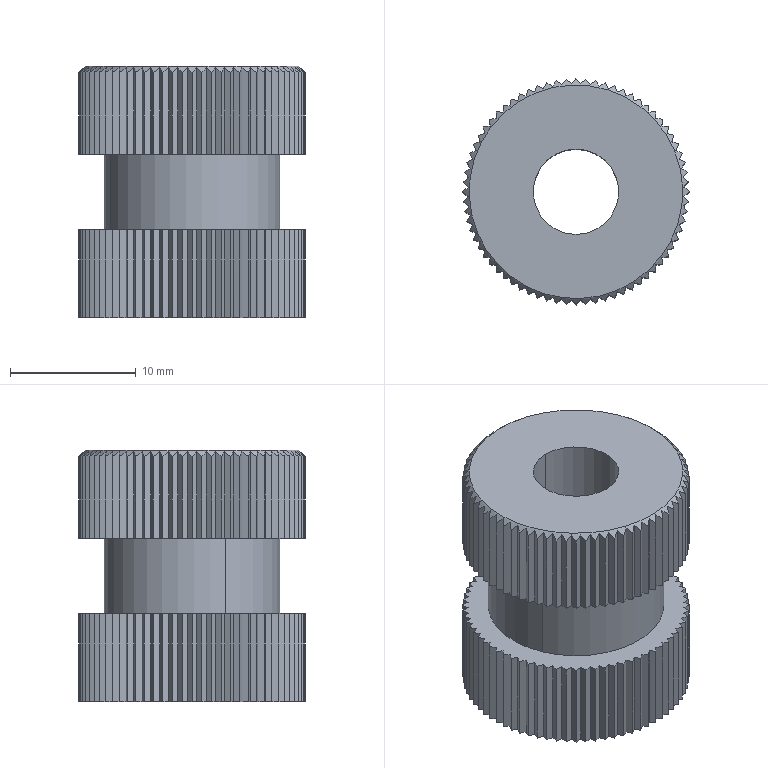Part | SolidWorks | features BaseBody 1 | 1 solid | 298 faces | box 18.005 x 18.005 x 20 mm | volume 3583 mm3 | plane 292 | cylinder 4 | cone 2 | commonest cylinder face diameters 6.8 x2 14 x2